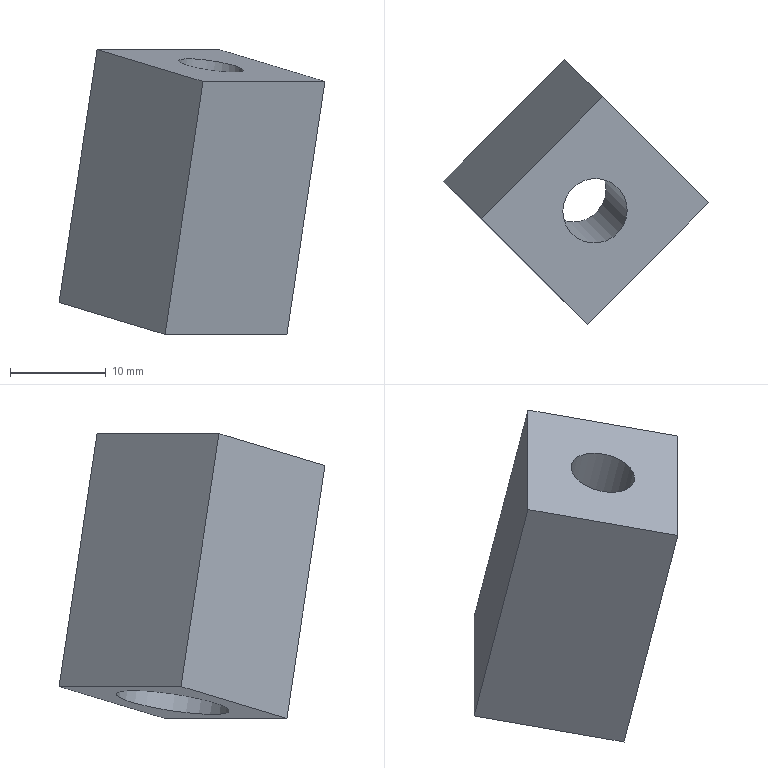Part | STEP file | gslz 2016.10.28-13_id1562_x_t | 1 solid | 9 faces | box 27.764 x 27.764 x 29.737 mm | volume 5874 mm3 | plane 7 | cylinder 2 | commonest cylinder face diameters 6.8 x1 12 x1
STEP:
#1=CARTESIAN_POINT('',(0.,0.,0.));
#2=DIRECTION('',(0.,0.,1.));
#3=DIRECTION('',(1.,0.,0.));
#4=AXIS2_PLACEMENT_3D('',#1,#2,#3);
#5=CARTESIAN_POINT('',(1037.927,286.05,-38.857));
#6=VERTEX_POINT('',#5);
#7=CARTESIAN_POINT('',(1034.564,286.013,-38.357));
#8=DIRECTION('',(-0.147,0.147,-0.9781));
#9=DIRECTION('',(0.9891,0.01093,-0.147));
#10=AXIS2_PLACEMENT_3D('',#7,#8,#9);
#11=CIRCLE('',#10,3.4);
#12=CARTESIAN_POINT('',(1054.25,305.659,-38.363));
#13=DIRECTION('',(0.147,-0.147,0.9781));
#14=DIRECTION('',(0.9891,0.01093,-0.147));
#15=AXIS2_PLACEMENT_3D('',#12,#13,#14);
#16=PLANE('',#15);
#17=CARTESIAN_POINT('',(-16.286,-19.645));
#18=CARTESIAN_POINT('',(-16.286,-25.534));
#19=CARTESIAN_POINT('',(-21.386,-22.59));
#20=CARTESIAN_POINT('',(-26.486,-19.645));
#21=CARTESIAN_POINT('',(-21.386,-16.701));
#22=CARTESIAN_POINT('',(-16.286,-13.756));
#23=CARTESIAN_POINT('',(-16.286,-19.645));
#24=(BOUNDED_CURVE()B_SPLINE_CURVE(2,(#17,#18,#19,#20,#21,#22,#23),.UNSPECIFIED.,.T.,.F.)B_SPLINE_CURVE_WITH_KNOTS((1,2,2,2,2,1),(-2.094,0.,2.094,4.189,6.283,8.378),.UNSPECIFIED.)CURVE()GEOMETRIC_REPRESENTATION_ITEM()RATIONAL_B_SPLINE_CURVE((1.,0.5,1.,0.5,1.,0.5,1.))REPRESENTATION_ITEM(''));
#25=(GEOMETRIC_REPRESENTATION_CONTEXT(2)PARAMETRIC_REPRESENTATION_CONTEXT()REPRESENTATION_CONTEXT('',''));
#26=DEFINITIONAL_REPRESENTATION('',(#24),#25);
#27=PCURVE('',#16,#26);
#28=CARTESIAN_POINT('',(1036.769,283.808,-23.685));
#29=DIRECTION('',(0.147,-0.147,0.9781));
#30=DIRECTION('',(0.9891,0.01093,-0.147));
#31=AXIS2_PLACEMENT_3D('',#28,#29,#30);
#32=CYLINDRICAL_SURFACE('',#31,3.4);
#33=CARTESIAN_POINT('',(6.283,-15.));
#34=DIRECTION('',(-1.,0.));
#35=VECTOR('',#34,1.);
#36=LINE('',#33,#35);
#37=(GEOMETRIC_REPRESENTATION_CONTEXT(2)PARAMETRIC_REPRESENTATION_CONTEXT()REPRESENTATION_CONTEXT('',''));
#38=DEFINITIONAL_REPRESENTATION('',(#36),#37);
#39=PCURVE('',#32,#38);
#40=SURFACE_CURVE('',#11,(#27,#39),.PCURVE_S1.);
#41=EDGE_CURVE('',#6,#6,#40,.T.);
#42=ORIENTED_EDGE('',*,*,#41,.T.);
#43=EDGE_LOOP('',(#42));
#44=FACE_BOUND('',#43,.T.);
#45=CARTESIAN_POINT('',(1046.461,286.844,-40.02));
#46=VERTEX_POINT('',#45);
#47=CARTESIAN_POINT('',(1033.734,274.116,-40.02));
#48=VERTEX_POINT('',#47);
#49=CARTESIAN_POINT('',(1048.583,288.965,-40.02));
#50=DIRECTION('',(-0.7071,-0.7071,0.));
#51=VECTOR('',#50,1.);
#52=LINE('',#49,#51);
#53=CARTESIAN_POINT('',(-5.544,-16.817));
#54=DIRECTION('',(-0.7071,-0.7071));
#55=VECTOR('',#54,1.);
#56=LINE('',#53,#55);
#57=(GEOMETRIC_REPRESENTATION_CONTEXT(2)PARAMETRIC_REPRESENTATION_CONTEXT()REPRESENTATION_CONTEXT('',''));
#58=DEFINITIONAL_REPRESENTATION('',(#56),#57);
#59=PCURVE('',#16,#58);
#60=CARTESIAN_POINT('',(1045.275,292.273,-62.028));
#61=DIRECTION('',(-0.6917,0.6917,0.2079));
#62=DIRECTION('',(-0.7071,-0.7071,0.));
#63=AXIS2_PLACEMENT_3D('',#60,#61,#62);
#64=PLANE('',#63);
#65=CARTESIAN_POINT('',(0.,22.5));
#66=DIRECTION('',(1.,0.));
#67=VECTOR('',#66,1.);
#68=LINE('',#65,#67);
#69=(GEOMETRIC_REPRESENTATION_CONTEXT(2)PARAMETRIC_REPRESENTATION_CONTEXT()REPRESENTATION_CONTEXT('',''));
#70=DEFINITIONAL_REPRESENTATION('',(#68),#69);
#71=PCURVE('',#64,#70);
#72=SURFACE_CURVE('',#52,(#59,#71),.PCURVE_S1.);
#73=EDGE_CURVE('',#46,#48,#72,.T.);
#74=ORIENTED_EDGE('',*,*,#73,.F.);
#75=CARTESIAN_POINT('',(1035.395,297.91,-36.693));
#76=VERTEX_POINT('',#75);
#77=CARTESIAN_POINT('',(1040.928,292.377,-38.357));
#78=DIRECTION('',(0.6917,-0.6917,-0.2079));
#79=VECTOR('',#78,1.);
#80=LINE('',#77,#79);
#81=CARTESIAN_POINT('',(-13.322,-13.281));
#82=DIRECTION('',(0.7071,-0.7071));
#83=VECTOR('',#82,1.);
#84=LINE('',#81,#83);
#85=(GEOMETRIC_REPRESENTATION_CONTEXT(2)PARAMETRIC_REPRESENTATION_CONTEXT()REPRESENTATION_CONTEXT('',''));
#86=DEFINITIONAL_REPRESENTATION('',(#84),#85);
#87=PCURVE('',#16,#86);
#88=CARTESIAN_POINT('',(1037.62,295.685,-60.365));
#89=DIRECTION('',(-0.7071,-0.7071,0.));
#90=DIRECTION('',(0.6917,-0.6917,-0.2079));
#91=AXIS2_PLACEMENT_3D('',#88,#89,#90);
#92=PLANE('',#91);
#93=CARTESIAN_POINT('',(0.,22.5));
#94=DIRECTION('',(1.,0.));
#95=VECTOR('',#94,1.);
#96=LINE('',#93,#95);
#97=(GEOMETRIC_REPRESENTATION_CONTEXT(2)PARAMETRIC_REPRESENTATION_CONTEXT()REPRESENTATION_CONTEXT('',''));
#98=DEFINITIONAL_REPRESENTATION('',(#96),#97);
#99=PCURVE('',#92,#98);
#100=SURFACE_CURVE('',#80,(#87,#99),.PCURVE_S1.);
#101=EDGE_CURVE('',#76,#46,#100,.T.);
#102=ORIENTED_EDGE('',*,*,#101,.F.);
#103=CARTESIAN_POINT('',(1022.667,285.182,-36.693));
#104=VERTEX_POINT('',#103);
#105=CARTESIAN_POINT('',(1037.516,300.032,-36.693));
#106=DIRECTION('',(-0.7071,-0.7071,0.));
#107=VECTOR('',#106,1.);
#108=LINE('',#105,#107);
#109=CARTESIAN_POINT('',(-16.858,-5.503));
#110=DIRECTION('',(-0.7071,-0.7071));
#111=VECTOR('',#110,1.);
#112=LINE('',#109,#111);
#113=(GEOMETRIC_REPRESENTATION_CONTEXT(2)PARAMETRIC_REPRESENTATION_CONTEXT()REPRESENTATION_CONTEXT('',''));
#114=DEFINITIONAL_REPRESENTATION('',(#112),#113);
#115=PCURVE('',#16,#114);
#116=CARTESIAN_POINT('',(1034.208,303.34,-58.702));
#117=DIRECTION('',(-0.6917,0.6917,0.2079));
#118=DIRECTION('',(-0.7071,-0.7071,0.));
#119=AXIS2_PLACEMENT_3D('',#116,#117,#118);
#120=PLANE('',#119);
#121=CARTESIAN_POINT('',(0.,22.5));
#122=DIRECTION('',(1.,0.));
#123=VECTOR('',#122,1.);
#124=LINE('',#121,#123);
#125=(GEOMETRIC_REPRESENTATION_CONTEXT(2)PARAMETRIC_REPRESENTATION_CONTEXT()REPRESENTATION_CONTEXT('',''));
#126=DEFINITIONAL_REPRESENTATION('',(#124),#125);
#127=PCURVE('',#120,#126);
#128=SURFACE_CURVE('',#108,(#115,#127),.PCURVE_S1.);
#129=EDGE_CURVE('',#76,#104,#128,.T.);
#130=ORIENTED_EDGE('',*,*,#129,.T.);
#131=CARTESIAN_POINT('',(1028.22,279.629,-38.363));
#132=DIRECTION('',(0.6917,-0.6917,-0.2079));
#133=VECTOR('',#132,1.);
#134=LINE('',#131,#133);
#135=CARTESIAN_POINT('',(-26.03,-26.03));
#136=DIRECTION('',(0.7071,-0.7071));
#137=VECTOR('',#136,1.);
#138=LINE('',#135,#137);
#139=(GEOMETRIC_REPRESENTATION_CONTEXT(2)PARAMETRIC_REPRESENTATION_CONTEXT()REPRESENTATION_CONTEXT('',''));
#140=DEFINITIONAL_REPRESENTATION('',(#138),#139);
#141=PCURVE('',#16,#140);
#142=CARTESIAN_POINT('',(1029.964,277.885,-26.761));
#143=DIRECTION('',(0.7071,0.7071,0.));
#144=DIRECTION('',(-0.6917,0.6917,0.2079));
#145=AXIS2_PLACEMENT_3D('',#142,#143,#144);
#146=PLANE('',#145);
#147=CARTESIAN_POINT('',(0.,-11.861));
#148=DIRECTION('',(-1.,0.));
#149=VECTOR('',#148,1.);
#150=LINE('',#147,#149);
#151=(GEOMETRIC_REPRESENTATION_CONTEXT(2)PARAMETRIC_REPRESENTATION_CONTEXT()REPRESENTATION_CONTEXT('',''));
#152=DEFINITIONAL_REPRESENTATION('',(#150),#151);
#153=PCURVE('',#146,#152);
#154=SURFACE_CURVE('',#134,(#141,#153),.PCURVE_S1.);
#155=EDGE_CURVE('',#104,#48,#154,.T.);
#156=ORIENTED_EDGE('',*,*,#155,.T.);
#157=EDGE_LOOP('',(#74,#102,#130,#156));
#158=FACE_BOUND('',#157,.T.);
#159=ADVANCED_FACE('',(#44,#158),#16,.T.);
#160=CARTESIAN_POINT('',(1042.492,290.813,-66.43));
#161=VERTEX_POINT('',#160);
#162=CARTESIAN_POINT('',(1029.764,278.085,-66.43));
#163=VERTEX_POINT('',#162);
#164=CARTESIAN_POINT('',(1044.613,292.935,-66.43));
#165=DIRECTION('',(-0.7071,-0.7071,0.));
#166=VECTOR('',#165,1.);
#167=LINE('',#164,#166);
#168=CARTESIAN_POINT('',(0.,-4.5));
#169=DIRECTION('',(1.,0.));
#170=VECTOR('',#169,1.);
#171=LINE('',#168,#170);
#172=(GEOMETRIC_REPRESENTATION_CONTEXT(2)PARAMETRIC_REPRESENTATION_CONTEXT()REPRESENTATION_CONTEXT('',''));
#173=DEFINITIONAL_REPRESENTATION('',(#171),#172);
#174=PCURVE('',#64,#173);
#175=CARTESIAN_POINT('',(1039.08,298.468,-64.767));
#176=DIRECTION('',(0.147,-0.147,0.9781));
#177=DIRECTION('',(0.9891,0.01093,-0.147));
#178=AXIS2_PLACEMENT_3D('',#175,#176,#177);
#179=PLANE('',#178);
#180=CARTESIAN_POINT('',(5.657,-5.657));
#181=DIRECTION('',(-0.7071,-0.7071));
#182=VECTOR('',#181,1.);
#183=LINE('',#180,#182);
#184=(GEOMETRIC_REPRESENTATION_CONTEXT(2)PARAMETRIC_REPRESENTATION_CONTEXT()REPRESENTATION_CONTEXT('',''));
#185=DEFINITIONAL_REPRESENTATION('',(#183),#184);
#186=PCURVE('',#179,#185);
#187=SURFACE_CURVE('',#167,(#174,#186),.PCURVE_S1.);
#188=EDGE_CURVE('',#161,#163,#187,.T.);
#189=ORIENTED_EDGE('',*,*,#188,.F.);
#190=CARTESIAN_POINT('',(1043.154,290.152,-62.028));
#191=DIRECTION('',(0.147,-0.147,0.9781));
#192=VECTOR('',#191,1.);
#193=LINE('',#190,#192);
#194=CARTESIAN_POINT('',(3.,0.));
#195=DIRECTION('',(0.,1.));
#196=VECTOR('',#195,1.);
#197=LINE('',#194,#196);
#198=(GEOMETRIC_REPRESENTATION_CONTEXT(2)PARAMETRIC_REPRESENTATION_CONTEXT()REPRESENTATION_CONTEXT('',''));
#199=DEFINITIONAL_REPRESENTATION('',(#197),#198);
#200=PCURVE('',#64,#199);
#201=CARTESIAN_POINT('',(8.,0.));
#202=DIRECTION('',(0.,1.));
#203=VECTOR('',#202,1.);
#204=LINE('',#201,#203);
#205=(GEOMETRIC_REPRESENTATION_CONTEXT(2)PARAMETRIC_REPRESENTATION_CONTEXT()REPRESENTATION_CONTEXT('',''));
#206=DEFINITIONAL_REPRESENTATION('',(#204),#205);
#207=PCURVE('',#92,#206);
#208=SURFACE_CURVE('',#193,(#200,#207),.PCURVE_S1.);
#209=EDGE_CURVE('',#161,#46,#208,.T.);
#210=ORIENTED_EDGE('',*,*,#209,.T.);
#211=ORIENTED_EDGE('',*,*,#73,.T.);
#212=CARTESIAN_POINT('',(1030.426,277.424,-62.028));
#213=DIRECTION('',(0.147,-0.147,0.9781));
#214=VECTOR('',#213,1.);
#215=LINE('',#212,#214);
#216=CARTESIAN_POINT('',(21.,0.));
#217=DIRECTION('',(0.,1.));
#218=VECTOR('',#217,1.);
#219=LINE('',#216,#218);
#220=(GEOMETRIC_REPRESENTATION_CONTEXT(2)PARAMETRIC_REPRESENTATION_CONTEXT()REPRESENTATION_CONTEXT('',''));
#221=DEFINITIONAL_REPRESENTATION('',(#219),#220);
#222=PCURVE('',#64,#221);
#223=CARTESIAN_POINT('',(-7.971,-34.361));
#224=DIRECTION('',(0.,1.));
#225=VECTOR('',#224,1.);
#226=LINE('',#223,#225);
#227=(GEOMETRIC_REPRESENTATION_CONTEXT(2)PARAMETRIC_REPRESENTATION_CONTEXT()REPRESENTATION_CONTEXT('',''));
#228=DEFINITIONAL_REPRESENTATION('',(#226),#227);
#229=PCURVE('',#146,#228);
#230=SURFACE_CURVE('',#215,(#222,#229),.PCURVE_S1.);
#231=EDGE_CURVE('',#163,#48,#230,.T.);
#232=ORIENTED_EDGE('',*,*,#231,.F.);
#233=EDGE_LOOP('',(#189,#210,#211,#232));
#234=FACE_BOUND('',#233,.T.);
#235=ADVANCED_FACE('',(#234),#64,.F.);
#236=CARTESIAN_POINT('',(1036.529,290.048,-65.649));
#237=VERTEX_POINT('',#236);
#238=CARTESIAN_POINT('',(1030.595,289.983,-64.767));
#239=DIRECTION('',(0.147,-0.147,0.9781));
#240=DIRECTION('',(0.9891,0.01093,-0.147));
#241=AXIS2_PLACEMENT_3D('',#238,#239,#240);
#242=CIRCLE('',#241,6.);
#243=CARTESIAN_POINT('',(-8.485,-8.485));
#244=DIRECTION('',(1.,0.));
#245=AXIS2_PLACEMENT_2D('',#243,#244);
#246=CIRCLE('',#245,6.);
#247=(GEOMETRIC_REPRESENTATION_CONTEXT(2)PARAMETRIC_REPRESENTATION_CONTEXT()REPRESENTATION_CONTEXT('',''));
#248=DEFINITIONAL_REPRESENTATION('',(#246),#247);
#249=PCURVE('',#179,#248);
#250=CARTESIAN_POINT('',(1029.419,291.159,-72.592));
#251=DIRECTION('',(0.147,-0.147,0.9781));
#252=DIRECTION('',(0.9891,0.01093,-0.147));
#253=AXIS2_PLACEMENT_3D('',#250,#251,#252);
#254=CYLINDRICAL_SURFACE('',#253,6.);
#255=CARTESIAN_POINT('',(0.,8.));
#256=DIRECTION('',(1.,0.));
#257=VECTOR('',#256,1.);
#258=LINE('',#255,#257);
#259=(GEOMETRIC_REPRESENTATION_CONTEXT(2)PARAMETRIC_REPRESENTATION_CONTEXT()REPRESENTATION_CONTEXT('',''));
#260=DEFINITIONAL_REPRESENTATION('',(#258),#259);
#261=PCURVE('',#254,#260);
#262=SURFACE_CURVE('',#242,(#249,#261),.PCURVE_S1.);
#263=EDGE_CURVE('',#237,#237,#262,.T.);
#264=ORIENTED_EDGE('',*,*,#263,.T.);
#265=EDGE_LOOP('',(#264));
#266=FACE_BOUND('',#265,.T.);
#267=CARTESIAN_POINT('',(1031.426,301.88,-63.103));
#268=VERTEX_POINT('',#267);
#269=CARTESIAN_POINT('',(1036.959,296.347,-64.767));
#270=DIRECTION('',(-0.6917,0.6917,0.2079));
#271=VECTOR('',#270,1.);
#272=LINE('',#269,#271);
#273=CARTESIAN_POINT('',(-2.121,-2.121));
#274=DIRECTION('',(-0.7071,0.7071));
#275=VECTOR('',#274,1.);
#276=LINE('',#273,#275);
#277=(GEOMETRIC_REPRESENTATION_CONTEXT(2)PARAMETRIC_REPRESENTATION_CONTEXT()REPRESENTATION_CONTEXT('',''));
#278=DEFINITIONAL_REPRESENTATION('',(#276),#277);
#279=PCURVE('',#179,#278);
#280=CARTESIAN_POINT('',(0.,-4.5));
#281=DIRECTION('',(-1.,0.));
#282=VECTOR('',#281,1.);
#283=LINE('',#280,#282);
#284=(GEOMETRIC_REPRESENTATION_CONTEXT(2)PARAMETRIC_REPRESENTATION_CONTEXT()REPRESENTATION_CONTEXT('',''));
#285=DEFINITIONAL_REPRESENTATION('',(#283),#284);
#286=PCURVE('',#92,#285);
#287=SURFACE_CURVE('',#272,(#279,#286),.PCURVE_S1.);
#288=EDGE_CURVE('',#161,#268,#287,.T.);
#289=ORIENTED_EDGE('',*,*,#288,.F.);
#290=ORIENTED_EDGE('',*,*,#188,.T.);
#291=CARTESIAN_POINT('',(1018.698,289.152,-63.103));
#292=VERTEX_POINT('',#291);
#293=CARTESIAN_POINT('',(1024.251,283.599,-64.773));
#294=DIRECTION('',(-0.6917,0.6917,0.2079));
#295=VECTOR('',#294,1.);
#296=LINE('',#293,#295);
#297=CARTESIAN_POINT('',(-14.829,-14.87));
#298=DIRECTION('',(-0.7071,0.7071));
#299=VECTOR('',#298,1.);
#300=LINE('',#297,#299);
#301=(GEOMETRIC_REPRESENTATION_CONTEXT(2)PARAMETRIC_REPRESENTATION_CONTEXT()REPRESENTATION_CONTEXT('',''));
#302=DEFINITIONAL_REPRESENTATION('',(#300),#301);
#303=PCURVE('',#179,#302);
#304=CARTESIAN_POINT('',(0.,-38.861));
#305=DIRECTION('',(1.,0.));
#306=VECTOR('',#305,1.);
#307=LINE('',#304,#306);
#308=(GEOMETRIC_REPRESENTATION_CONTEXT(2)PARAMETRIC_REPRESENTATION_CONTEXT()REPRESENTATION_CONTEXT('',''));
#309=DEFINITIONAL_REPRESENTATION('',(#307),#308);
#310=PCURVE('',#146,#309);
#311=SURFACE_CURVE('',#296,(#303,#310),.PCURVE_S1.);
#312=EDGE_CURVE('',#163,#292,#311,.T.);
#313=ORIENTED_EDGE('',*,*,#312,.T.);
#314=CARTESIAN_POINT('',(1033.547,304.001,-63.103));
#315=DIRECTION('',(-0.7071,-0.7071,0.));
#316=VECTOR('',#315,1.);
#317=LINE('',#314,#316);
#318=CARTESIAN_POINT('',(-5.657,5.657));
#319=DIRECTION('',(-0.7071,-0.7071));
#320=VECTOR('',#319,1.);
#321=LINE('',#318,#320);
#322=(GEOMETRIC_REPRESENTATION_CONTEXT(2)PARAMETRIC_REPRESENTATION_CONTEXT()REPRESENTATION_CONTEXT('',''));
#323=DEFINITIONAL_REPRESENTATION('',(#321),#322);
#324=PCURVE('',#179,#323);
#325=CARTESIAN_POINT('',(0.,-4.5));
#326=DIRECTION('',(1.,0.));
#327=VECTOR('',#326,1.);
#328=LINE('',#325,#327);
#329=(GEOMETRIC_REPRESENTATION_CONTEXT(2)PARAMETRIC_REPRESENTATION_CONTEXT()REPRESENTATION_CONTEXT('',''));
#330=DEFINITIONAL_REPRESENTATION('',(#328),#329);
#331=PCURVE('',#120,#330);
#332=SURFACE_CURVE('',#317,(#324,#331),.PCURVE_S1.);
#333=EDGE_CURVE('',#268,#292,#332,.T.);
#334=ORIENTED_EDGE('',*,*,#333,.F.);
#335=EDGE_LOOP('',(#289,#290,#313,#334));
#336=FACE_BOUND('',#335,.T.);
#337=ADVANCED_FACE('',(#266,#336),#179,.F.);
#338=ORIENTED_EDGE('',*,*,#129,.F.);
#339=CARTESIAN_POINT('',(1032.087,301.218,-58.702));
#340=DIRECTION('',(0.147,-0.147,0.9781));
#341=VECTOR('',#340,1.);
#342=LINE('',#339,#341);
#343=CARTESIAN_POINT('',(3.,0.));
#344=DIRECTION('',(0.,1.));
#345=VECTOR('',#344,1.);
#346=LINE('',#343,#345);
#347=(GEOMETRIC_REPRESENTATION_CONTEXT(2)PARAMETRIC_REPRESENTATION_CONTEXT()REPRESENTATION_CONTEXT('',''));
#348=DEFINITIONAL_REPRESENTATION('',(#346),#347);
#349=PCURVE('',#120,#348);
#350=CARTESIAN_POINT('',(-8.,0.));
#351=DIRECTION('',(0.,1.));
#352=VECTOR('',#351,1.);
#353=LINE('',#350,#352);
#354=(GEOMETRIC_REPRESENTATION_CONTEXT(2)PARAMETRIC_REPRESENTATION_CONTEXT()REPRESENTATION_CONTEXT('',''));
#355=DEFINITIONAL_REPRESENTATION('',(#353),#354);
#356=PCURVE('',#92,#355);
#357=SURFACE_CURVE('',#342,(#349,#356),.PCURVE_S1.);
#358=EDGE_CURVE('',#268,#76,#357,.T.);
#359=ORIENTED_EDGE('',*,*,#358,.F.);
#360=ORIENTED_EDGE('',*,*,#333,.T.);
#361=CARTESIAN_POINT('',(1019.359,288.49,-58.702));
#362=DIRECTION('',(0.147,-0.147,0.9781));
#363=VECTOR('',#362,1.);
#364=LINE('',#361,#363);
#365=CARTESIAN_POINT('',(21.,0.));
#366=DIRECTION('',(0.,1.));
#367=VECTOR('',#366,1.);
#368=LINE('',#365,#367);
#369=(GEOMETRIC_REPRESENTATION_CONTEXT(2)PARAMETRIC_REPRESENTATION_CONTEXT()REPRESENTATION_CONTEXT('',''));
#370=DEFINITIONAL_REPRESENTATION('',(#368),#369);
#371=PCURVE('',#120,#370);
#372=CARTESIAN_POINT('',(8.029,-34.361));
#373=DIRECTION('',(0.,1.));
#374=VECTOR('',#373,1.);
#375=LINE('',#372,#374);
#376=(GEOMETRIC_REPRESENTATION_CONTEXT(2)PARAMETRIC_REPRESENTATION_CONTEXT()REPRESENTATION_CONTEXT('',''));
#377=DEFINITIONAL_REPRESENTATION('',(#375),#376);
#378=PCURVE('',#146,#377);
#379=SURFACE_CURVE('',#364,(#371,#378),.PCURVE_S1.);
#380=EDGE_CURVE('',#292,#104,#379,.T.);
#381=ORIENTED_EDGE('',*,*,#380,.T.);
#382=EDGE_LOOP('',(#338,#359,#360,#381));
#383=FACE_BOUND('',#382,.T.);
#384=ADVANCED_FACE('',(#383),#120,.T.);
#385=ORIENTED_EDGE('',*,*,#101,.T.);
#386=ORIENTED_EDGE('',*,*,#209,.F.);
#387=ORIENTED_EDGE('',*,*,#288,.T.);
#388=ORIENTED_EDGE('',*,*,#358,.T.);
#389=EDGE_LOOP('',(#385,#386,#387,#388));
#390=FACE_BOUND('',#389,.T.);
#391=ADVANCED_FACE('',(#390),#92,.F.);
#392=ORIENTED_EDGE('',*,*,#155,.F.);
#393=ORIENTED_EDGE('',*,*,#380,.F.);
#394=ORIENTED_EDGE('',*,*,#312,.F.);
#395=ORIENTED_EDGE('',*,*,#231,.T.);
#396=EDGE_LOOP('',(#392,#393,#394,#395));
#397=FACE_BOUND('',#396,.T.);
#398=ADVANCED_FACE('',(#397),#146,.F.);
#399=CARTESIAN_POINT('',(1035.722,288.256,-53.529));
#400=VERTEX_POINT('',#399);
#401=CARTESIAN_POINT('',(1032.359,288.218,-53.029));
#402=DIRECTION('',(-0.147,0.147,-0.9781));
#403=DIRECTION('',(0.9891,0.01093,-0.147));
#404=AXIS2_PLACEMENT_3D('',#401,#402,#403);
#405=CIRCLE('',#404,3.4);
#406=CARTESIAN_POINT('',(6.283,-30.));
#407=DIRECTION('',(-1.,0.));
#408=VECTOR('',#407,1.);
#409=LINE('',#406,#408);
#410=(GEOMETRIC_REPRESENTATION_CONTEXT(2)PARAMETRIC_REPRESENTATION_CONTEXT()REPRESENTATION_CONTEXT('',''));
#411=DEFINITIONAL_REPRESENTATION('',(#409),#410);
#412=PCURVE('',#32,#411);
#413=CARTESIAN_POINT('',(1032.359,288.218,-53.029));
#414=DIRECTION('',(0.147,-0.147,0.9781));
#415=DIRECTION('',(0.9891,0.01093,-0.147));
#416=AXIS2_PLACEMENT_3D('',#413,#414,#415);
#417=PLANE('',#416);
#418=CARTESIAN_POINT('',(3.4,0.));
#419=CARTESIAN_POINT('',(3.4,-5.889));
#420=CARTESIAN_POINT('',(-1.7,-2.944));
#421=CARTESIAN_POINT('',(-6.8,0.));
#422=CARTESIAN_POINT('',(-1.7,2.944));
#423=CARTESIAN_POINT('',(3.4,5.889));
#424=CARTESIAN_POINT('',(3.4,0.));
#425=(BOUNDED_CURVE()B_SPLINE_CURVE(2,(#418,#419,#420,#421,#422,#423,#424),.UNSPECIFIED.,.T.,.F.)B_SPLINE_CURVE_WITH_KNOTS((1,2,2,2,2,1),(-2.094,0.,2.094,4.189,6.283,8.378),.UNSPECIFIED.)CURVE()GEOMETRIC_REPRESENTATION_ITEM()RATIONAL_B_SPLINE_CURVE((1.,0.5,1.,0.5,1.,0.5,1.))REPRESENTATION_ITEM(''));
#426=(GEOMETRIC_REPRESENTATION_CONTEXT(2)PARAMETRIC_REPRESENTATION_CONTEXT()REPRESENTATION_CONTEXT('',''));
#427=DEFINITIONAL_REPRESENTATION('',(#425),#426);
#428=PCURVE('',#417,#427);
#429=SURFACE_CURVE('',#405,(#412,#428),.PCURVE_S1.);
#430=EDGE_CURVE('',#400,#400,#429,.T.);
#431=ORIENTED_EDGE('',*,*,#430,.F.);
#432=CARTESIAN_POINT('',(1035.722,288.256,-53.529));
#433=CARTESIAN_POINT('',(1037.927,286.05,-38.857));
#434=B_SPLINE_CURVE_WITH_KNOTS('',1,(#432,#433),.UNSPECIFIED.,.F.,.F.,(2,2),(-30.,-15.),.PIECEWISE_BEZIER_KNOTS.);
#435=CARTESIAN_POINT('',(6.283,0.));
#436=DIRECTION('',(0.,1.));
#437=VECTOR('',#436,1.);
#438=LINE('',#435,#437);
#439=(GEOMETRIC_REPRESENTATION_CONTEXT(2)PARAMETRIC_REPRESENTATION_CONTEXT()REPRESENTATION_CONTEXT('',''));
#440=DEFINITIONAL_REPRESENTATION('',(#438),#439);
#441=PCURVE('',#32,#440);
#442=CARTESIAN_POINT('',(0.,0.));
#443=DIRECTION('',(0.,1.));
#444=VECTOR('',#443,1.);
#445=LINE('',#442,#444);
#446=(GEOMETRIC_REPRESENTATION_CONTEXT(2)PARAMETRIC_REPRESENTATION_CONTEXT()REPRESENTATION_CONTEXT('',''));
#447=DEFINITIONAL_REPRESENTATION('',(#445),#446);
#448=PCURVE('',#32,#447);
#449=SEAM_CURVE('',#434,(#441,#448),.PCURVE_S1.);
#450=EDGE_CURVE('',#400,#6,#449,.T.);
#451=ORIENTED_EDGE('',*,*,#450,.T.);
#452=ORIENTED_EDGE('',*,*,#41,.T.);
#453=ORIENTED_EDGE('',*,*,#450,.F.);
#454=EDGE_LOOP('',(#431,#451,#452,#453));
#455=FACE_BOUND('',#454,.F.);
#456=ADVANCED_FACE('',(#455),#32,.F.);
#457=ORIENTED_EDGE('',*,*,#430,.F.);
#458=EDGE_LOOP('',(#457));
#459=FACE_BOUND('',#458,.T.);
#460=CARTESIAN_POINT('',(1038.293,288.284,-53.911));
#461=VERTEX_POINT('',#460);
#462=CARTESIAN_POINT('',(1032.359,288.218,-53.029));
#463=DIRECTION('',(-0.147,0.147,-0.9781));
#464=DIRECTION('',(0.9891,0.01093,-0.147));
#465=AXIS2_PLACEMENT_3D('',#462,#463,#464);
#466=CIRCLE('',#465,6.);
#467=CARTESIAN_POINT('',(6.,0.));
#468=CARTESIAN_POINT('',(6.,-10.392));
#469=CARTESIAN_POINT('',(-3.,-5.196));
#470=CARTESIAN_POINT('',(-12.,0.));
#471=CARTESIAN_POINT('',(-3.,5.196));
#472=CARTESIAN_POINT('',(6.,10.392));
#473=CARTESIAN_POINT('',(6.,0.));
#474=(BOUNDED_CURVE()B_SPLINE_CURVE(2,(#467,#468,#469,#470,#471,#472,#473),.UNSPECIFIED.,.T.,.F.)B_SPLINE_CURVE_WITH_KNOTS((1,2,2,2,2,1),(-2.094,0.,2.094,4.189,6.283,8.378),.UNSPECIFIED.)CURVE()GEOMETRIC_REPRESENTATION_ITEM()RATIONAL_B_SPLINE_CURVE((1.,0.5,1.,0.5,1.,0.5,1.))REPRESENTATION_ITEM(''));
#475=(GEOMETRIC_REPRESENTATION_CONTEXT(2)PARAMETRIC_REPRESENTATION_CONTEXT()REPRESENTATION_CONTEXT('',''));
#476=DEFINITIONAL_REPRESENTATION('',(#474),#475);
#477=PCURVE('',#417,#476);
#478=CARTESIAN_POINT('',(6.283,20.));
#479=DIRECTION('',(-1.,0.));
#480=VECTOR('',#479,1.);
#481=LINE('',#478,#480);
#482=(GEOMETRIC_REPRESENTATION_CONTEXT(2)PARAMETRIC_REPRESENTATION_CONTEXT()REPRESENTATION_CONTEXT('',''));
#483=DEFINITIONAL_REPRESENTATION('',(#481),#482);
#484=PCURVE('',#254,#483);
#485=SURFACE_CURVE('',#466,(#477,#484),.PCURVE_S1.);
#486=EDGE_CURVE('',#461,#461,#485,.T.);
#487=ORIENTED_EDGE('',*,*,#486,.T.);
#488=EDGE_LOOP('',(#487));
#489=FACE_BOUND('',#488,.T.);
#490=ADVANCED_FACE('',(#459,#489),#417,.F.);
#491=ORIENTED_EDGE('',*,*,#486,.T.);
#492=CARTESIAN_POINT('',(1036.529,290.048,-65.649));
#493=CARTESIAN_POINT('',(1038.293,288.284,-53.911));
#494=B_SPLINE_CURVE_WITH_KNOTS('',1,(#492,#493),.UNSPECIFIED.,.F.,.F.,(2,2),(8.,20.),.PIECEWISE_BEZIER_KNOTS.);
#495=CARTESIAN_POINT('',(0.,0.));
#496=DIRECTION('',(0.,1.));
#497=VECTOR('',#496,1.);
#498=LINE('',#495,#497);
#499=(GEOMETRIC_REPRESENTATION_CONTEXT(2)PARAMETRIC_REPRESENTATION_CONTEXT()REPRESENTATION_CONTEXT('',''));
#500=DEFINITIONAL_REPRESENTATION('',(#498),#499);
#501=PCURVE('',#254,#500);
#502=CARTESIAN_POINT('',(6.283,0.));
#503=DIRECTION('',(0.,1.));
#504=VECTOR('',#503,1.);
#505=LINE('',#502,#504);
#506=(GEOMETRIC_REPRESENTATION_CONTEXT(2)PARAMETRIC_REPRESENTATION_CONTEXT()REPRESENTATION_CONTEXT('',''));
#507=DEFINITIONAL_REPRESENTATION('',(#505),#506);
#508=PCURVE('',#254,#507);
#509=SEAM_CURVE('',#494,(#501,#508),.PCURVE_S1.);
#510=EDGE_CURVE('',#237,#461,#509,.T.);
#511=ORIENTED_EDGE('',*,*,#510,.F.);
#512=ORIENTED_EDGE('',*,*,#263,.T.);
#513=ORIENTED_EDGE('',*,*,#510,.T.);
#514=EDGE_LOOP('',(#491,#511,#512,#513));
#515=FACE_BOUND('',#514,.F.);
#516=ADVANCED_FACE('',(#515),#254,.F.);
#517=CLOSED_SHELL('',(#159,#235,#337,#384,#391,#398,#456,#490,#516));
#518=MANIFOLD_SOLID_BREP('',#517);
#519=(LENGTH_UNIT()NAMED_UNIT(*)SI_UNIT(.MILLI.,.METRE.));
#520=UNCERTAINTY_MEASURE_WITH_UNIT(LENGTH_MEASURE(0.000002),#519,'','');
#521=(NAMED_UNIT(*)PLANE_ANGLE_UNIT()SI_UNIT($,.RADIAN.));
#522=(NAMED_UNIT(*)SI_UNIT($,.STERADIAN.)SOLID_ANGLE_UNIT());
#523=(GEOMETRIC_REPRESENTATION_CONTEXT(3)GLOBAL_UNCERTAINTY_ASSIGNED_CONTEXT((#520))GLOBAL_UNIT_ASSIGNED_CONTEXT((#519,#521,#522))REPRESENTATION_CONTEXT('',''));
#524=ADVANCED_BREP_SHAPE_REPRESENTATION('',(#4,#518),#523);